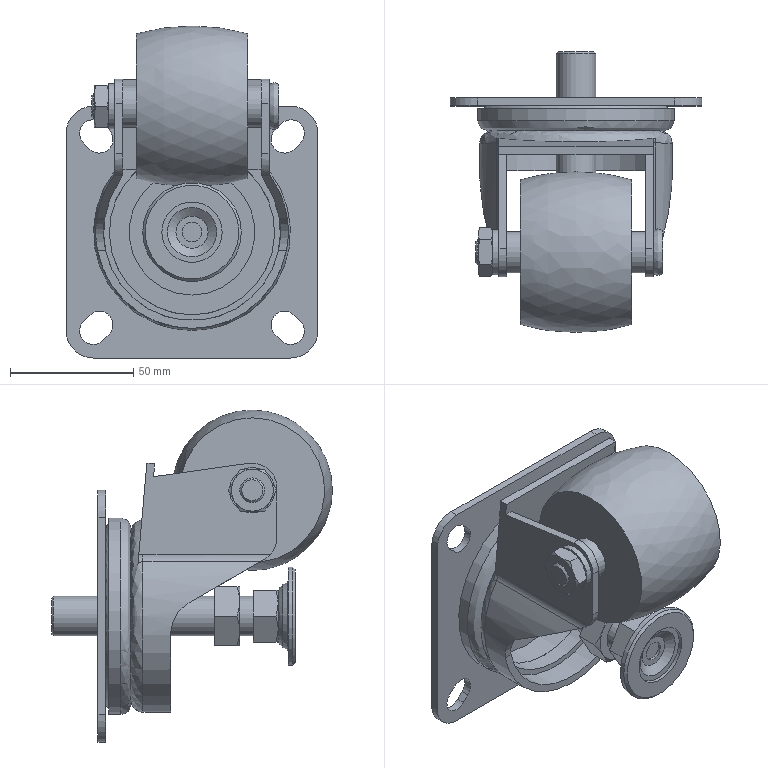Part | NX | features CMAS65-F 12 | 11 solids | 157 faces | box 102 x 113.8 x 134.5 mm | volume 246246 mm3 | plane 79 | cylinder 48 | cone 21 | spline 9 | commonest cylinder face diameters 11 x8 20 x6 10 x5 16 x4 22 x4 30 x4